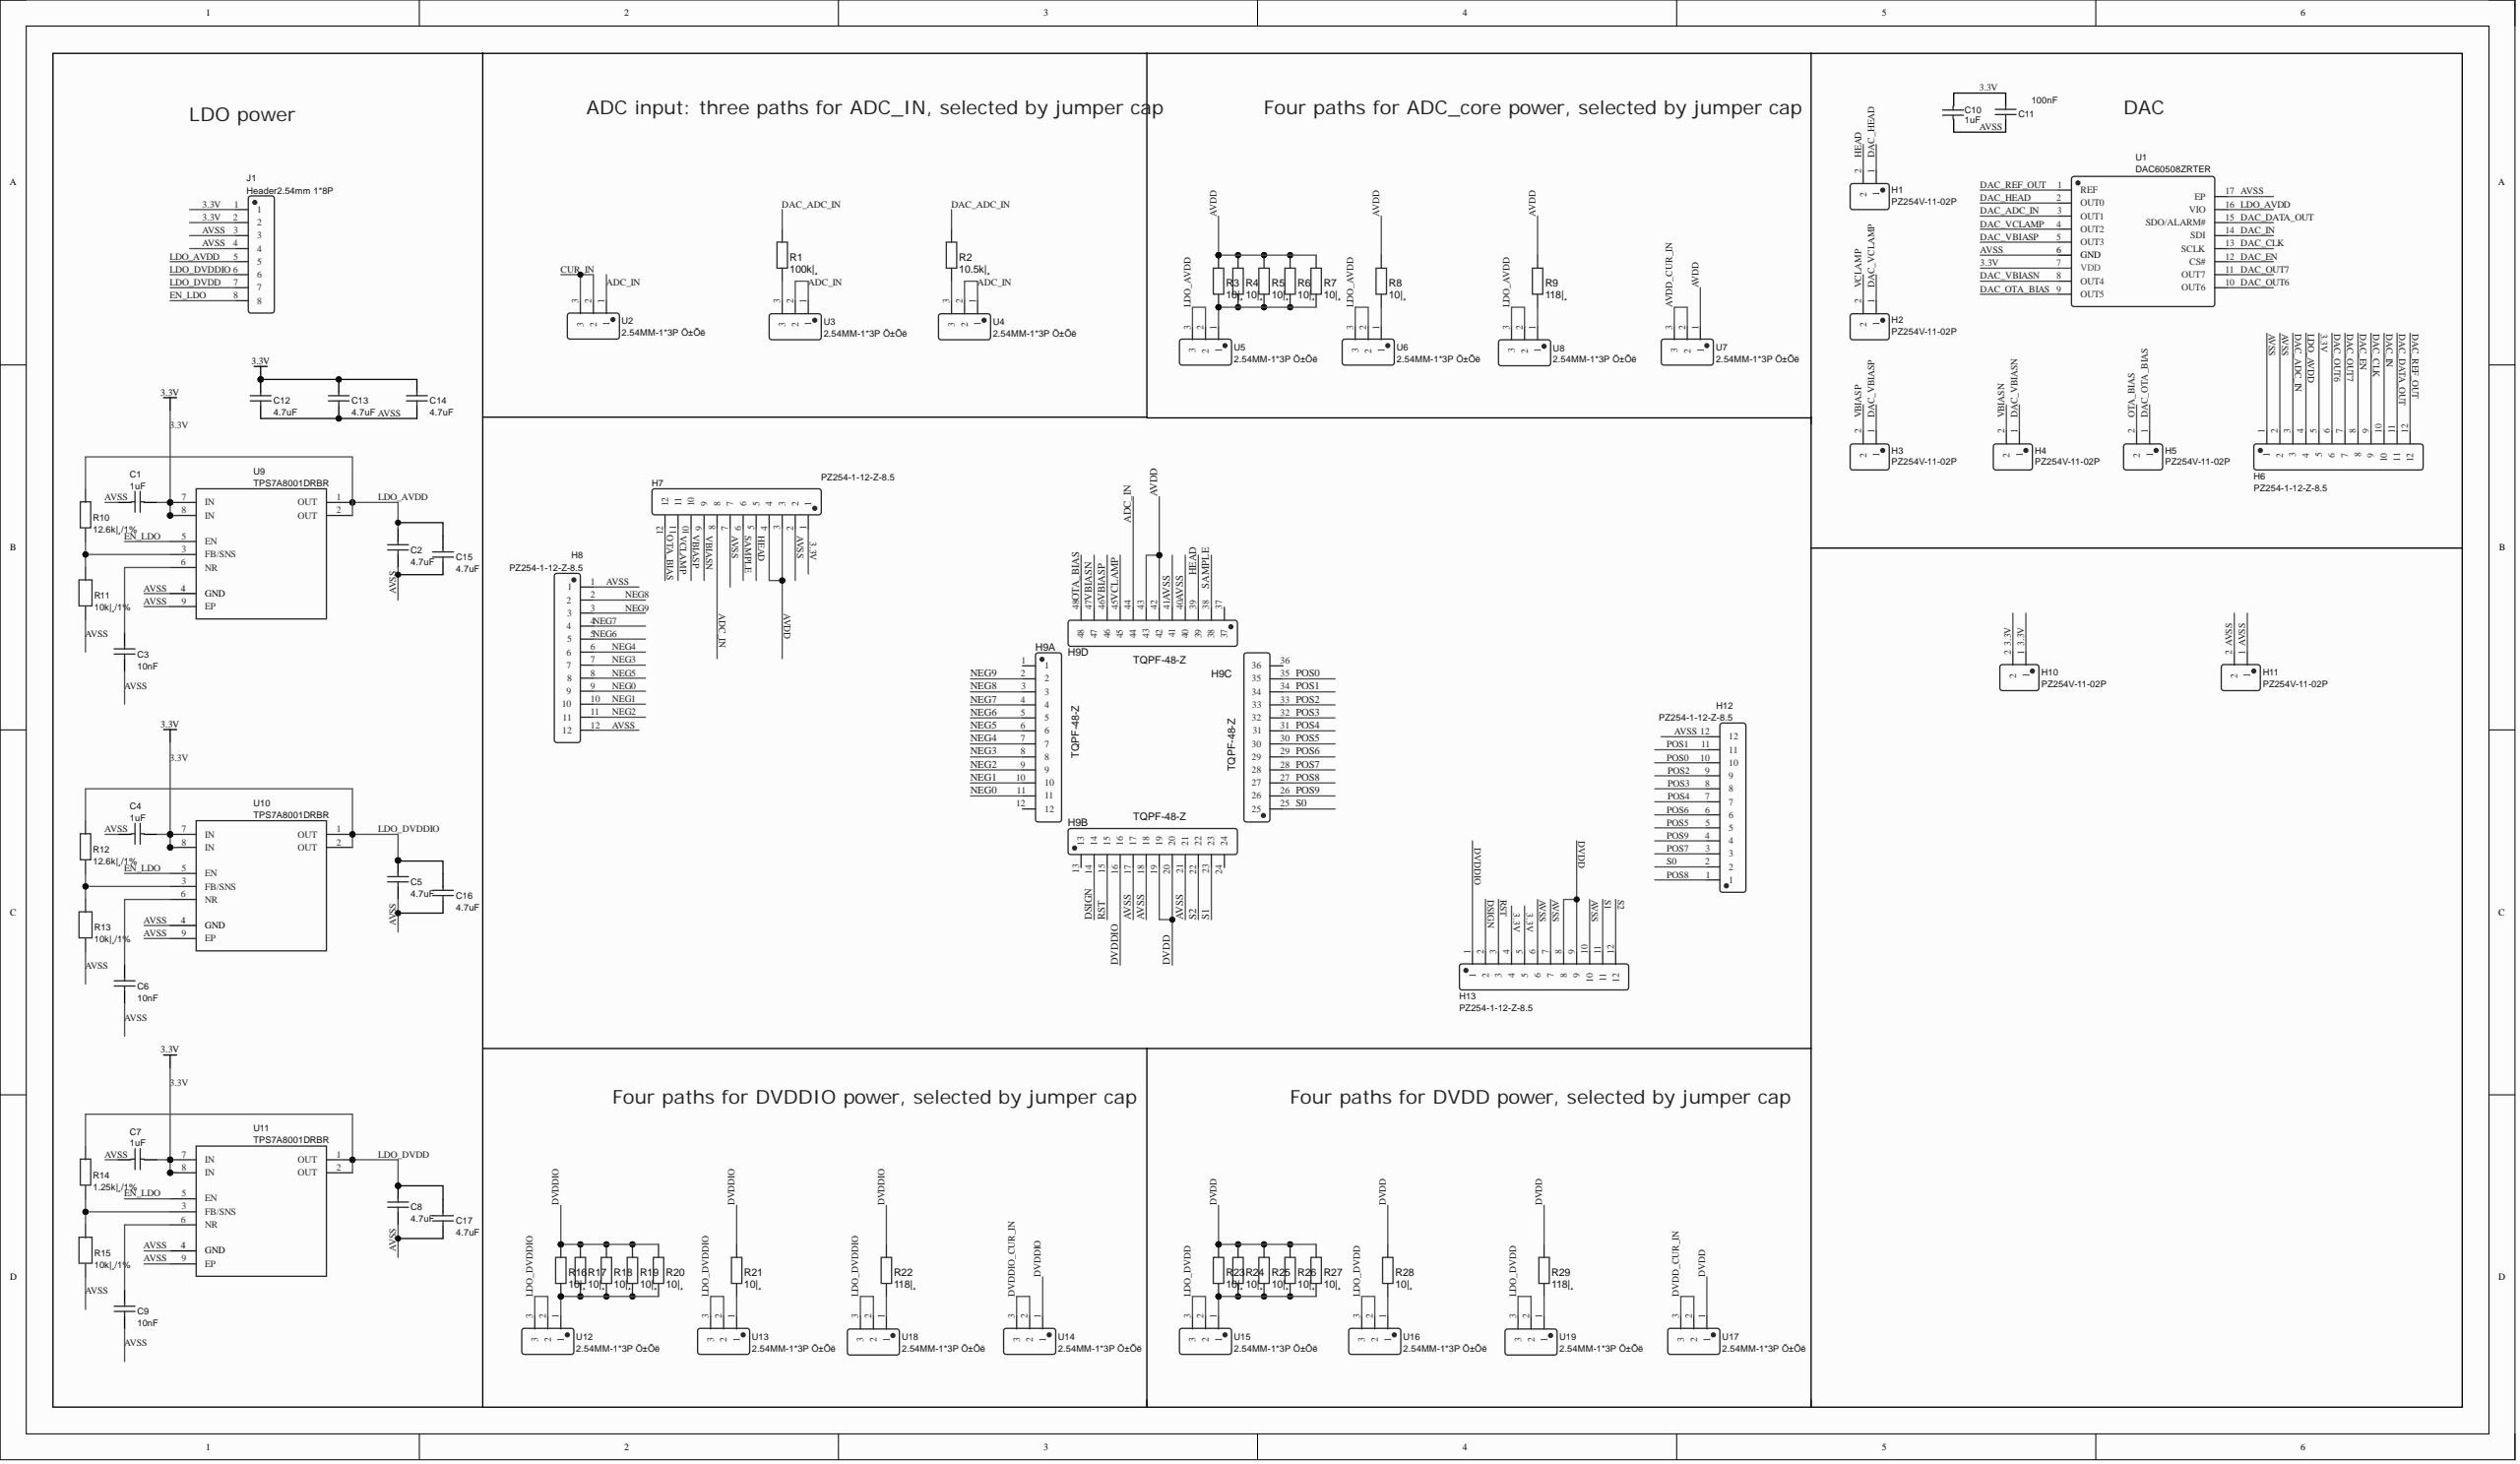Circuit board | Altium Designer | 79 parts | 75 nets
Bill of materials:
Comment,Description,Designator,Footprint,LibRef,Quantity
"1uF","","C1, C4, C7, C10","C0603","1uF","4"
"4.7uF","","C2, C5, C8, C12, C13, C14, C15, C16, C17","C0603","4.7uF","9"
"10nF","","C3, C6, C9","C0603","10nF","3"
"100nF","","C11","C0603","10nF","1"
"PZ254V-11-02P","","H1, H2, H3, H4, H5, H10, H11","HDR-TH_2P-P2.54-V-M","PZ254V-11-02P","7"
"PZ254-1-12-Z-8.5","","H6, H7, H8, H12, H13","HDR-TH_12P-P2.54-V-M","PZ254-1-12-Z-8.5","5"
"TQPF-48-Z","","H9","TQPF-48-Z","PZ254-1-12-Z-8.5","1"
"Header2.54mm 1*8P","","J1","HDR-TH_8P-P2.54-V-M","Header2.54mm 1*8P","1"
"100k|¸","","R1","R0805","100k|¸","1"
"10.5k|¸","","R2","R0603","10.5k|¸","1"
"10|¸","","R3, R4, R5, R6, R7, R8, R16, R17, R18, R19, R20, R21, R23, R24, R25, R26, R27, R28","R1206","10|¸","18"
"118|¸","","R9, R22, R29","R0603","118|¸","3"
"12.6k|¸/1%","","R10, R12","R0603","12.6k|¸/1%","2"
"10k|¸/1%","","R11, R13, R15","R0603","10k|¸/1%","3"
"1.25k|¸/1%","","R14","R0805","1.25k|¸/1%","1"
"DAC60508ZRTER","","U1","WQFN-16_L3.0-W3.0-P0.50-BL-EP0.8","DAC60508ZRTER","1"
"2.54MM-1*3P 直针","","U2, U3, U4, U5, U6, U7, U8, U12, U13, U14, U15, U16, U17, U18, U19","HDR-TH_3P-P2.54-V-M-1","2.54MM-1*3P 直针","15"
"TPS7A8001DRBR","","U9, U10, U11","VSON-8_L3.0-W3.0-P0.65-TL-EP","TPS7A8001DRBR","3"
Netlist (Protel format):
[
C1
C0603
1uF



]
[
C2
C0603
4.7uF



]
[
C3
C0603
10nF



]
[
C4
C0603
1uF



]
[
C5
C0603
4.7uF



]
[
C6
C0603
10nF



]
[
C7
C0603
1uF



]
[
C8
C0603
4.7uF



]
[
C9
C0603
10nF



]
[
C10
C0603
1uF



]
[
C11
C0603
100nF



]
[
C12
C0603
4.7uF



]
[
C13
C0603
4.7uF



]
[
C14
C0603
4.7uF



]
[
C15
C0603
4.7uF



]
[
C16
C0603
4.7uF



]
[
C17
C0603
4.7uF



]
[
H1
HDR-TH_2P-P2.54-V-M
PZ254V-11-02P



]
[
H2
HDR-TH_2P-P2.54-V-M
PZ254V-11-02P



]
[
H3
HDR-TH_2P-P2.54-V-M
PZ254V-11-02P



]
[
H4
HDR-TH_2P-P2.54-V-M
PZ254V-11-02P



]
[
H5
HDR-TH_2P-P2.54-V-M
PZ254V-11-02P



]
[
H6
HDR-TH_12P-P2.54-V-M
PZ254-1-12-Z-8.5



]
[
H7
HDR-TH_12P-P2.54-V-M
PZ254-1-12-Z-8.5



]
[
H8
HDR-TH_12P-P2.54-V-M
PZ254-1-12-Z-8.5



]
[
H9
TQPF-48-Z
TQPF-48-Z



]
[
H10
HDR-TH_2P-P2.54-V-M
PZ254V-11-02P



]
[
H11
HDR-TH_2P-P2.54-V-M
PZ254V-11-02P



]
[
H12
HDR-TH_12P-P2.54-V-M
PZ254-1-12-Z-8.5



]
[
H13
HDR-TH_12P-P2.54-V-M
PZ254-1-12-Z-8.5



]
[
J1
HDR-TH_8P-P2.54-V-M
Header2.54mm 1*8P



]
[
R1
R0805
100k|¸



]
[
R2
R0603
10.5k|¸



]
[
R3
R1206
10|¸



]
[
R4
R1206
10|¸



]
[
R5
R1206
10|¸



]
[
R6
R1206
10|¸



]
[
R7
R1206
10|¸



]
[
R8
R1206
10|¸



]
[
R9
R0603
118|¸



]
[
R10
R0603
12.6k|¸/1%



]
[
R11
R0603
10k|¸/1%



]
[
R12
R0603
12.6k|¸/1%



]
[
R13
R0603
10k|¸/1%



]
[
R14
R0805
1.25k|¸/1%



]
[
R15
R0603
10k|¸/1%



]
[
R16
R1206
10|¸



]
[
R17
R1206
10|¸



]
[
R18
R1206
10|¸



]
[
R19
R1206
10|¸



]
[
R20
R1206
10|¸



]
[
R21
R1206
10|¸



]
[
R22
R0603
118|¸



]
[
R23
R1206
10|¸



]
[
R24
R1206
10|¸



]
[
R25
R1206
10|¸



]
[
R26
R1206
10|¸



]
[
R27
R1206
10|¸



]
[
R28
R1206
10|¸



]
[
R29
R0603
118|¸



]
[
U1
WQFN-16_L3.0-W3.0-P0.50-BL-EP0.8
DAC60508ZRTER



]
[
U2
HDR-TH_3P-P2.54-V-M-1
2.54MM-1*3P 直针



]
[
U3
HDR-TH_3P-P2.54-V-M-1
2.54MM-1*3P 直针



]
[
U4
HDR-TH_3P-P2.54-V-M-1
2.54MM-1*3P 直针



]
[
U5
HDR-TH_3P-P2.54-V-M-1
2.54MM-1*3P 直针



]
[
U6
HDR-TH_3P-P2.54-V-M-1
2.54MM-1*3P 直针



]
[
U7
HDR-TH_3P-P2.54-V-M-1
2.54MM-1*3P 直针



]
[
U8
HDR-TH_3P-P2.54-V-M-1
2.54MM-1*3P 直针



]
[
U9
VSON-8_L3.0-W3.0-P0.65-TL-EP
TPS7A8001DRBR



]
[
U10
VSON-8_L3.0-W3.0-P0.65-TL-EP
TPS7A8001DRBR



]
[
U11
VSON-8_L3.0-W3.0-P0.65-TL-EP
TPS7A8001DRBR



]
[
U12
HDR-TH_3P-P2.54-V-M-1
2.54MM-1*3P 直针



]
[
U13
HDR-TH_3P-P2.54-V-M-1
2.54MM-1*3P 直针



]
[
U14
HDR-TH_3P-P2.54-V-M-1
2.54MM-1*3P 直针



]
[
U15
HDR-TH_3P-P2.54-V-M-1
2.54MM-1*3P 直针



]
[
U16
HDR-TH_3P-P2.54-V-M-1
2.54MM-1*3P 直针



]
[
U17
HDR-TH_3P-P2.54-V-M-1
2.54MM-1*3P 直针



]
[
U18
HDR-TH_3P-P2.54-V-M-1
2.54MM-1*3P 直针



]
[
U19
HDR-TH_3P-P2.54-V-M-1
2.54MM-1*3P 直针



]
(
VCLAMP
H2-2
H7-11
H9-45
)
(
VBIASP
H3-2
H7-10
H9-46
)
(
VBIASN
H4-2
H7-9
H9-47
)
(
SAMPLE
H7-6
H9-38
)
(
S2
H9-22
H13-12
)
(
S1
H9-23
H13-11
)
(
S0
H9-25
H12-2
)
(
RST
H9-15
H13-3
)
(
POS9
H9-26
H12-4
)
(
POS8
H9-27
H12-1
)
(
POS7
H9-28
H12-3
)
(
POS6
H9-29
H12-6
)
(
POS5
H9-30
H12-5
)
(
POS4
H9-31
H12-7
)
(
POS3
H9-32
H12-8
)
(
POS2
H9-33
H12-9
)
(
POS1
H9-34
H12-11
)
(
POS0
H9-35
H12-10
)
(
OTA_BIAS
H5-2
H7-12
H9-48
)
(
NetR29_1
R29-1
U19-1
)
(
NetR28_1
R28-1
U16-1
)
(
NetR23_1
R23-1
R24-1
R25-1
R26-1
R27-1
U15-1
)
(
NetR22_1
R22-1
U18-1
)
(
NetR21_1
R21-1
U13-1
)
(
NetR16_1
R16-1
R17-1
R18-1
R19-1
R20-1
U12-1
)
(
NetR14_2
R14-2
R15-2
U11-3
)
(
NetR12_2
R12-2
R13-2
U10-3
)
(
NetR10_2
R10-2
R11-2
U9-3
)
(
NetR9_1
R9-1
U8-1
)
(
NetR8_1
R8-1
U6-1
)
(
NetR3_1
R3-1
R4-1
R5-1
R6-1
R7-1
U5-1
)
(
NetR2_1
R2-1
U4-3
)
(
NetR1_1
R1-1
U3-3
)
(
NetC9_2
C9-2
U11-6
)
(
NetC6_2
C6-2
U10-6
)
(
NetC3_2
C3-2
U9-6
)
(
NEG9
H8-3
H9-2
)
(
NEG8
H8-2
H9-3
)
(
NEG7
H8-4
H9-4
)
(
NEG6
H8-5
H9-5
)
(
NEG5
H8-8
H9-6
)
(
NEG4
H8-6
H9-7
)
(
NEG3
H8-7
H9-8
)
(
NEG2
H8-11
H9-9
)
(
NEG1
H8-10
H9-10
)
(
NEG0
H8-9
H9-11
)
(
LDO_DVDDIO
C5-2
C16-2
J1-6
R12-1
U10-1
U10-2
U12-2
U12-3
U13-2
U13-3
U18-2
U18-3
)
(
LDO_DVDD
C8-2
C17-2
J1-7
R14-1
U11-1
U11-2
U15-2
U15-3
U16-2
U16-3
U19-2
U19-3
)
(
LDO_AVDD
C2-2
C15-2
H6-4
J1-5
R10-1
U1-16
U5-2
U5-3
U6-2
U6-3
U8-2
U8-3
U9-1
U9-2
)
(
HEAD
H1-2
H7-5
H9-39
)
(
EN_LDO
J1-8
U9-5
U10-5
U11-5
)
(
DVDDIO_CUR_IN
U14-2
U14-3
)
(
DVDDIO
H9-16
H13-1
R16-2
R17-2
R18-2
R19-2
R20-2
R21-2
R22-2
U14-1
)
(
DVDD_CUR_IN
U17-2
U17-3
)
(
DVDD
H9-19
H9-20
H13-8
H13-9
R23-2
R24-2
R25-2
R26-2
R27-2
R28-2
R29-2
U17-1
)
(
DSIGN
H9-14
H13-2
)
(
DAC_VCLAMP
H2-1
U1-4
)
(
DAC_VBIASP
H3-1
U1-5
)
(
DAC_VBIASN
H4-1
U1-8
)
(
DAC_REF_OUT
H6-12
U1-1
)
(
DAC_OUT7
H6-7
U1-11
)
(
DAC_OUT6
H6-6
U1-10
)
(
DAC_OTA_BIAS
H5-1
U1-9
)
(
DAC_IN
H6-10
U1-14
)
(
DAC_HEAD
H1-1
U1-2
)
(
DAC_EN
H6-8
U1-12
)
(
DAC_DATA_OUT
H6-11
U1-15
)
(
DAC_CLK
H6-9
U1-13
)
(
DAC_ADC_IN
H6-3
R1-2
R2-2
U1-3
)
(
CUR_IN
U2-2
U2-3
)
(
AVSS
C1-2
C2-1
C3-1
C4-2
C5-1
C6-1
C7-2
C8-1
C9-1
C10-2
C11-1
C12-1
C13-1
C14-1
C15-1
C16-1
C17-1
H6-1
H6-2
H7-2
H7-7
H8-1
H8-12
H9-17
H9-18
H9-21
H9-40
H9-41
H11-1
H11-2
H12-12
H13-6
H13-7
H13-10
J1-3
J1-4
R11-1
R13-1
R15-1
U1-6
U1-17
U9-4
U9-9
U10-4
U10-9
U11-4
U11-9
)
(
AVDD_CUR_IN
U7-2
U7-3
)
(
AVDD
H7-3
H7-4
H9-42
H9-43
R3-2
R4-2
R5-2
R6-2
R7-2
R8-2
R9-2
U7-1
)
(
ADC_IN
H7-8
H9-44
U2-1
U3-1
U3-2
U4-1
U4-2
)
(
3.3V
C1-1
C4-1
C7-1
C10-1
C11-2
C12-2
C13-2
C14-2
H6-5
H7-1
H10-1
H10-2
H13-4
H13-5
J1-1
J1-2
U1-7
U9-7
U9-8
U10-7
U10-8
U11-7
U11-8
)